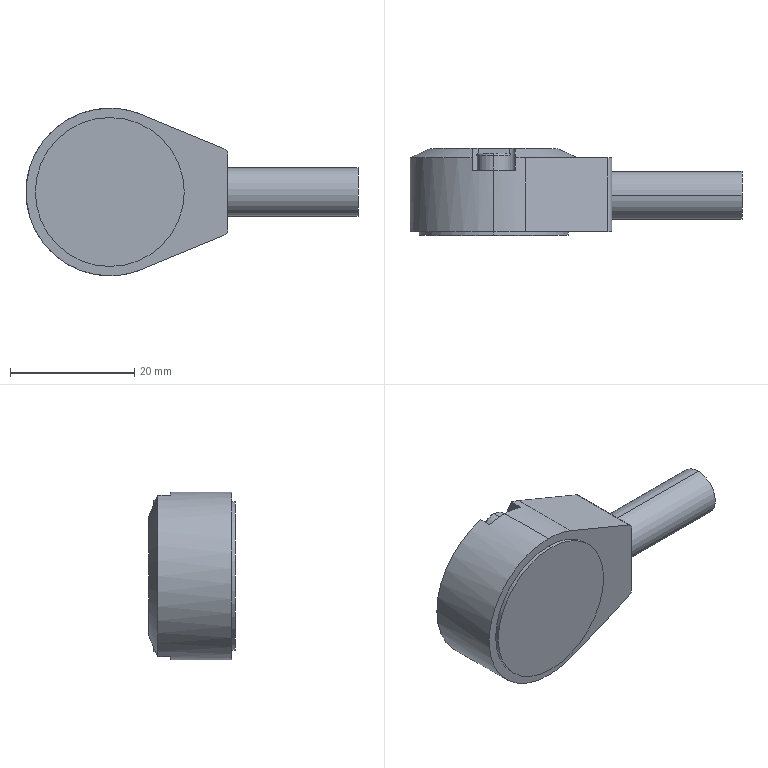Part | STEP file | OM-BHI62E-5RA-CC05AC33P-EPCR1201-2_Cable-1 | 1 solid | 41 faces | box 53.5 x 14 x 27 mm | volume 9959 mm3 | plane 18 | cylinder 17 | torus 4 | cone 2 | commonest cylinder face diameters 2 x6 5.5 x4 27 x3 7.8 x2 24 x2